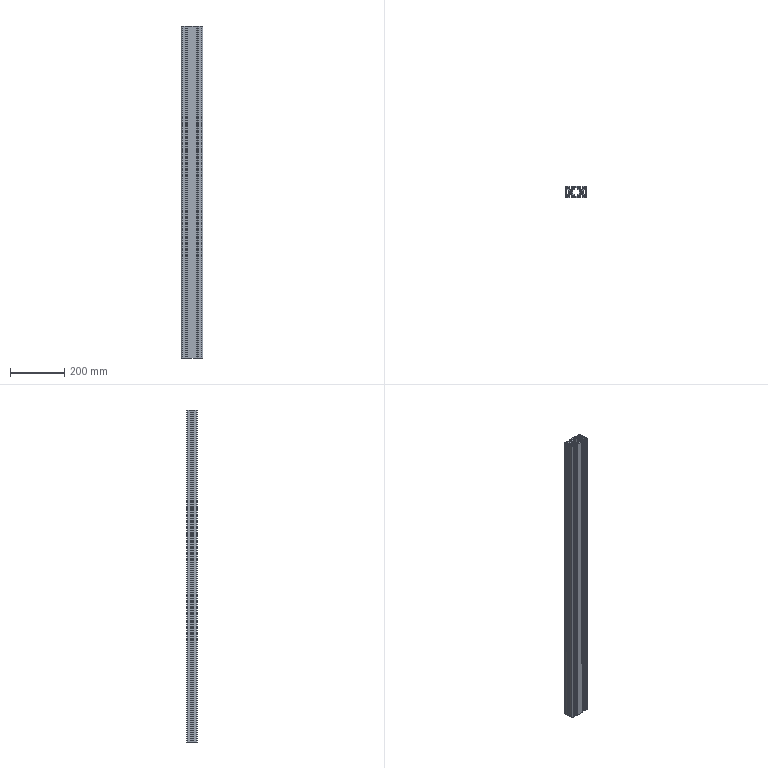Part | STEP file | HM-8-4080D-L1220 | 1 solid | 286 faces | box 80 x 40 x 1220 mm | volume 1475152 mm3 | plane 150 | cylinder 136 | commonest cylinder face diameters 0.6 x80 0.4 x36 6 x8 5 x4 6.8 x4 9 x4